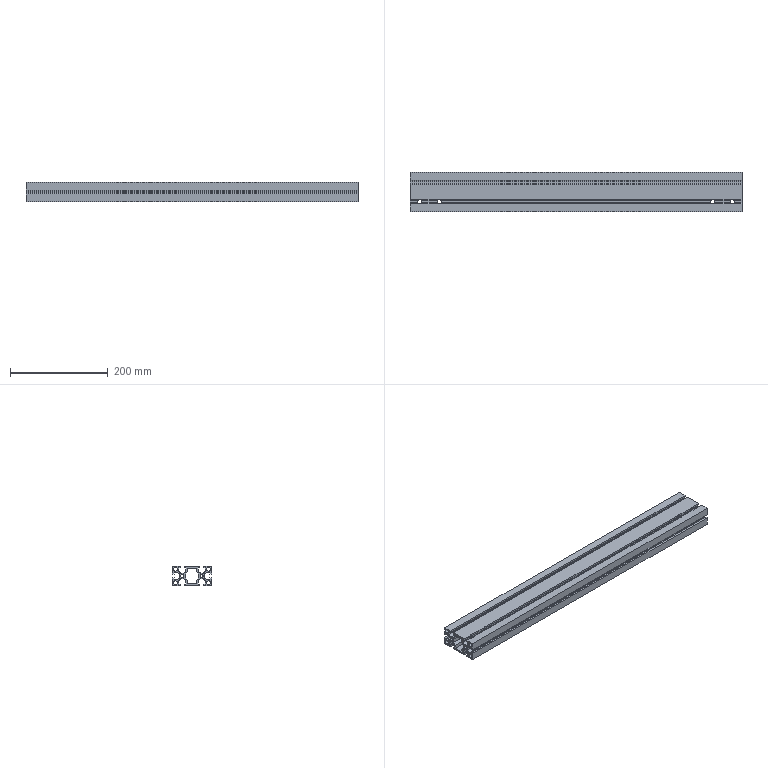Part | SolidWorks | features BaseBody 1 | 1 solid | 166 faces | box 680 x 80 x 40 mm | volume 834999 mm3 | plane 94 | cylinder 72 | commonest cylinder face diameters 10 x20 9 x16 14 x16 6.2 x12 8 x8